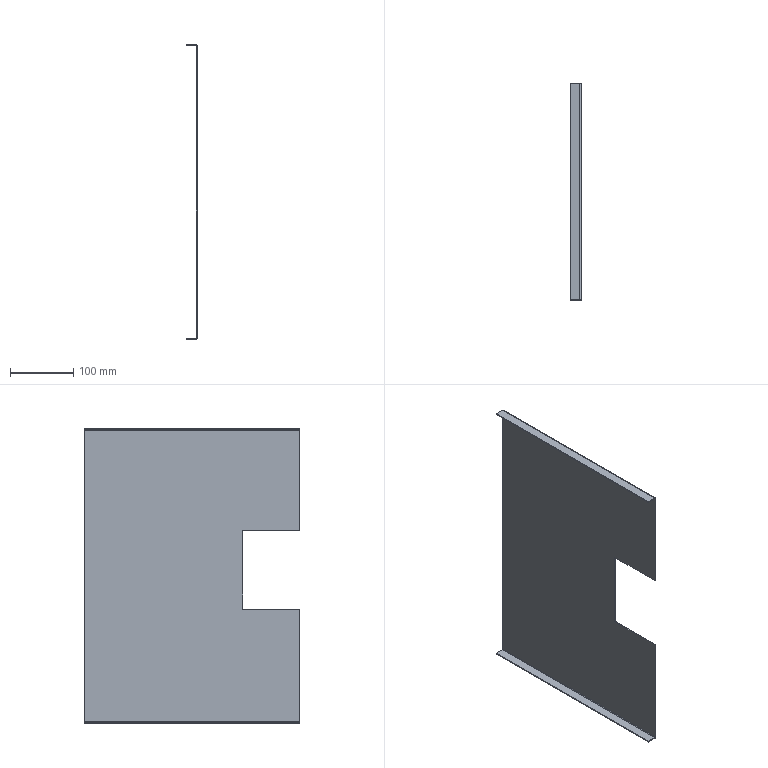Part | SolidWorks | features BaseBody 1 | 1 solid | 18 faces | box 16.5 x 340 x 464 mm | volume 234549 mm3 | plane 14 | cylinder 4 | commonest cylinder face diameters 1.473 x2 4.473 x2
STEP:
#1=CARTESIAN_POINT('',(0.,0.,-460.263));
#2=VERTEX_POINT('',#1);
#3=CARTESIAN_POINT('',(0.,0.,-282.737));
#4=VERTEX_POINT('',#3);
#5=CARTESIAN_POINT('',(0.,0.,0.));
#6=DIRECTION('',(0.,0.,1.));
#7=VECTOR('',#6,1000.);
#8=LINE('',#5,#7);
#9=EDGE_CURVE('',#2,#4,#8,.T.);
#10=ORIENTED_EDGE('',*,*,#9,.T.);
#11=CARTESIAN_POINT('',(0.,90.,-282.737));
#12=VERTEX_POINT('',#11);
#13=CARTESIAN_POINT('',(0.,340.,-282.737));
#14=DIRECTION('',(0.,1.,0.));
#15=VECTOR('',#14,1000.);
#16=LINE('',#13,#15);
#17=EDGE_CURVE('',#4,#12,#16,.T.);
#18=ORIENTED_EDGE('',*,*,#17,.T.);
#19=CARTESIAN_POINT('',(0.,90.,-158.737));
#20=VERTEX_POINT('',#19);
#21=CARTESIAN_POINT('',(0.,90.,0.));
#22=DIRECTION('',(0.,0.,1.));
#23=VECTOR('',#22,1000.);
#24=LINE('',#21,#23);
#25=EDGE_CURVE('',#12,#20,#24,.T.);
#26=ORIENTED_EDGE('',*,*,#25,.T.);
#27=CARTESIAN_POINT('',(0.,0.,-158.737));
#28=VERTEX_POINT('',#27);
#29=CARTESIAN_POINT('',(0.,340.,-158.737));
#30=DIRECTION('',(0.,-1.,0.));
#31=VECTOR('',#30,1000.);
#32=LINE('',#29,#31);
#33=EDGE_CURVE('',#20,#28,#32,.T.);
#34=ORIENTED_EDGE('',*,*,#33,.T.);
#35=CARTESIAN_POINT('',(0.,0.,-0.7366));
#36=VERTEX_POINT('',#35);
#37=CARTESIAN_POINT('',(0.,0.,0.));
#38=DIRECTION('',(0.,0.,1.));
#39=VECTOR('',#38,1000.);
#40=LINE('',#37,#39);
#41=EDGE_CURVE('',#28,#36,#40,.T.);
#42=ORIENTED_EDGE('',*,*,#41,.T.);
#43=CARTESIAN_POINT('',(0.,340.,-0.7366));
#44=VERTEX_POINT('',#43);
#45=CARTESIAN_POINT('',(0.,340.,-0.7366));
#46=DIRECTION('',(0.,1.,0.));
#47=VECTOR('',#46,1000.);
#48=LINE('',#45,#47);
#49=EDGE_CURVE('',#36,#44,#48,.T.);
#50=ORIENTED_EDGE('',*,*,#49,.T.);
#51=CARTESIAN_POINT('',(0.,340.,-460.263));
#52=VERTEX_POINT('',#51);
#53=CARTESIAN_POINT('',(0.,340.,0.));
#54=DIRECTION('',(0.,0.,-1.));
#55=VECTOR('',#54,1000.);
#56=LINE('',#53,#55);
#57=EDGE_CURVE('',#44,#52,#56,.T.);
#58=ORIENTED_EDGE('',*,*,#57,.T.);
#59=CARTESIAN_POINT('',(0.,340.,-460.263));
#60=DIRECTION('',(0.,-1.,0.));
#61=VECTOR('',#60,1000.);
#62=LINE('',#59,#61);
#63=EDGE_CURVE('',#52,#2,#62,.T.);
#64=ORIENTED_EDGE('',*,*,#63,.T.);
#65=EDGE_LOOP('',(#10,#18,#26,#34,#42,#50,#58,#64));
#66=FACE_OUTER_BOUND('',#65,.T.);
#67=CARTESIAN_POINT('',(0.,340.,0.));
#68=DIRECTION('',(-1.,0.,0.));
#69=DIRECTION('',(0.,0.,1.));
#70=AXIS2_PLACEMENT_3D('',#67,#68,#69);
#71=PLANE('',#70);
#72=ADVANCED_FACE('',(#66),#71,.T.);
#73=CARTESIAN_POINT('',(1.5,0.,-282.737));
#74=VERTEX_POINT('',#73);
#75=CARTESIAN_POINT('',(-8.5,0.,-282.737));
#76=DIRECTION('',(-1.,0.,0.));
#77=VECTOR('',#76,1000.);
#78=LINE('',#75,#77);
#79=EDGE_CURVE('',#74,#4,#78,.T.);
#80=ORIENTED_EDGE('',*,*,#79,.F.);
#81=CARTESIAN_POINT('',(1.5,90.,-282.737));
#82=VERTEX_POINT('',#81);
#83=CARTESIAN_POINT('',(1.5,0.,-282.737));
#84=DIRECTION('',(0.,-1.,0.));
#85=VECTOR('',#84,1000.);
#86=LINE('',#83,#85);
#87=EDGE_CURVE('',#82,#74,#86,.T.);
#88=ORIENTED_EDGE('',*,*,#87,.F.);
#89=CARTESIAN_POINT('',(-8.5,90.,-282.737));
#90=DIRECTION('',(1.,0.,0.));
#91=VECTOR('',#90,1000.);
#92=LINE('',#89,#91);
#93=EDGE_CURVE('',#12,#82,#92,.T.);
#94=ORIENTED_EDGE('',*,*,#93,.F.);
#95=ORIENTED_EDGE('',*,*,#17,.F.);
#96=EDGE_LOOP('',(#80,#88,#94,#95));
#97=FACE_OUTER_BOUND('',#96,.T.);
#98=CARTESIAN_POINT('',(-8.5,0.,-282.737));
#99=DIRECTION('',(0.,0.,-1.));
#100=DIRECTION('',(-1.,0.,0.));
#101=AXIS2_PLACEMENT_3D('',#98,#99,#100);
#102=PLANE('',#101);
#103=ADVANCED_FACE('',(#97),#102,.F.);
#104=ORIENTED_EDGE('',*,*,#9,.F.);
#105=CARTESIAN_POINT('',(-0.7366,0.,-461.));
#106=VERTEX_POINT('',#105);
#107=CARTESIAN_POINT('',(-0.7366,0.,-460.263));
#108=DIRECTION('',(0.,1.,0.));
#109=DIRECTION('',(0.,0.,-1.));
#110=AXIS2_PLACEMENT_3D('',#107,#108,#109);
#111=CIRCLE('',#110,0.7366);
#112=EDGE_CURVE('',#2,#106,#111,.T.);
#113=ORIENTED_EDGE('',*,*,#112,.T.);
#114=CARTESIAN_POINT('',(-15.,0.,-461.));
#115=VERTEX_POINT('',#114);
#116=CARTESIAN_POINT('',(0.,0.,-461.));
#117=DIRECTION('',(1.,0.,0.));
#118=VECTOR('',#117,1000.);
#119=LINE('',#116,#118);
#120=EDGE_CURVE('',#115,#106,#119,.T.);
#121=ORIENTED_EDGE('',*,*,#120,.F.);
#122=CARTESIAN_POINT('',(-15.,0.,-462.5));
#123=VERTEX_POINT('',#122);
#124=CARTESIAN_POINT('',(-15.,0.,-461.));
#125=DIRECTION('',(0.,0.,1.));
#126=VECTOR('',#125,1000.);
#127=LINE('',#124,#126);
#128=EDGE_CURVE('',#123,#115,#127,.T.);
#129=ORIENTED_EDGE('',*,*,#128,.F.);
#130=CARTESIAN_POINT('',(-0.7366,0.,-462.5));
#131=VERTEX_POINT('',#130);
#132=CARTESIAN_POINT('',(-0.7366,0.,-462.5));
#133=DIRECTION('',(1.,0.,0.));
#134=VECTOR('',#133,1000.);
#135=LINE('',#132,#134);
#136=EDGE_CURVE('',#123,#131,#135,.T.);
#137=ORIENTED_EDGE('',*,*,#136,.T.);
#138=CARTESIAN_POINT('',(1.5,0.,-460.263));
#139=VERTEX_POINT('',#138);
#140=CARTESIAN_POINT('',(-0.7366,0.,-460.263));
#141=DIRECTION('',(0.,1.,0.));
#142=DIRECTION('',(0.,0.,-1.));
#143=AXIS2_PLACEMENT_3D('',#140,#141,#142);
#144=CIRCLE('',#143,2.237);
#145=EDGE_CURVE('',#139,#131,#144,.T.);
#146=ORIENTED_EDGE('',*,*,#145,.F.);
#147=CARTESIAN_POINT('',(1.5,0.,-462.5));
#148=DIRECTION('',(0.,0.,1.));
#149=VECTOR('',#148,1000.);
#150=LINE('',#147,#149);
#151=EDGE_CURVE('',#139,#74,#150,.T.);
#152=ORIENTED_EDGE('',*,*,#151,.T.);
#153=ORIENTED_EDGE('',*,*,#79,.T.);
#154=EDGE_LOOP('',(#104,#113,#121,#129,#137,#146,#152,#153));
#155=FACE_OUTER_BOUND('',#154,.T.);
#156=CARTESIAN_POINT('',(-0.7366,0.,-462.5));
#157=DIRECTION('',(0.,-1.,0.));
#158=DIRECTION('',(0.,0.,-1.));
#159=AXIS2_PLACEMENT_3D('',#156,#157,#158);
#160=PLANE('',#159);
#161=ADVANCED_FACE('',(#155),#160,.T.);
#162=ORIENTED_EDGE('',*,*,#63,.F.);
#163=CARTESIAN_POINT('',(-0.7366,340.,-461.));
#164=VERTEX_POINT('',#163);
#165=CARTESIAN_POINT('',(-0.7366,340.,-460.263));
#166=DIRECTION('',(0.,-1.,0.));
#167=DIRECTION('',(0.,0.,-1.));
#168=AXIS2_PLACEMENT_3D('',#165,#166,#167);
#169=CIRCLE('',#168,0.7366);
#170=EDGE_CURVE('',#164,#52,#169,.T.);
#171=ORIENTED_EDGE('',*,*,#170,.F.);
#172=CARTESIAN_POINT('',(-0.7366,340.,-461.));
#173=DIRECTION('',(0.,1.,0.));
#174=VECTOR('',#173,1000.);
#175=LINE('',#172,#174);
#176=EDGE_CURVE('',#106,#164,#175,.T.);
#177=ORIENTED_EDGE('',*,*,#176,.F.);
#178=ORIENTED_EDGE('',*,*,#112,.F.);
#179=EDGE_LOOP('',(#162,#171,#177,#178));
#180=FACE_OUTER_BOUND('',#179,.T.);
#181=CARTESIAN_POINT('',(-0.7366,340.,-460.263));
#182=DIRECTION('',(0.,-1.,0.));
#183=DIRECTION('',(0.,0.,-1.));
#184=AXIS2_PLACEMENT_3D('',#181,#182,#183);
#185=CYLINDRICAL_SURFACE('',#184,0.7366);
#186=ADVANCED_FACE('',(#180),#185,.F.);
#187=CARTESIAN_POINT('',(1.5,340.,-0.7366));
#188=VERTEX_POINT('',#187);
#189=CARTESIAN_POINT('',(1.5,340.,-460.263));
#190=VERTEX_POINT('',#189);
#191=CARTESIAN_POINT('',(1.5,340.,1.5));
#192=DIRECTION('',(0.,0.,-1.));
#193=VECTOR('',#192,1000.);
#194=LINE('',#191,#193);
#195=EDGE_CURVE('',#188,#190,#194,.T.);
#196=ORIENTED_EDGE('',*,*,#195,.T.);
#197=CARTESIAN_POINT('',(-0.7366,340.,-462.5));
#198=VERTEX_POINT('',#197);
#199=CARTESIAN_POINT('',(-0.7366,340.,-460.263));
#200=DIRECTION('',(0.,-1.,0.));
#201=DIRECTION('',(0.,0.,-1.));
#202=AXIS2_PLACEMENT_3D('',#199,#200,#201);
#203=CIRCLE('',#202,2.237);
#204=EDGE_CURVE('',#198,#190,#203,.T.);
#205=ORIENTED_EDGE('',*,*,#204,.F.);
#206=CARTESIAN_POINT('',(-15.,340.,-462.5));
#207=VERTEX_POINT('',#206);
#208=CARTESIAN_POINT('',(1.5,340.,-462.5));
#209=DIRECTION('',(-1.,0.,0.));
#210=VECTOR('',#209,1000.);
#211=LINE('',#208,#210);
#212=EDGE_CURVE('',#198,#207,#211,.T.);
#213=ORIENTED_EDGE('',*,*,#212,.T.);
#214=CARTESIAN_POINT('',(-15.,340.,-461.));
#215=VERTEX_POINT('',#214);
#216=CARTESIAN_POINT('',(-15.,340.,-461.));
#217=DIRECTION('',(0.,0.,-1.));
#218=VECTOR('',#217,1000.);
#219=LINE('',#216,#218);
#220=EDGE_CURVE('',#215,#207,#219,.T.);
#221=ORIENTED_EDGE('',*,*,#220,.F.);
#222=CARTESIAN_POINT('',(0.,340.,-461.));
#223=DIRECTION('',(-1.,0.,0.));
#224=VECTOR('',#223,1000.);
#225=LINE('',#222,#224);
#226=EDGE_CURVE('',#164,#215,#225,.T.);
#227=ORIENTED_EDGE('',*,*,#226,.F.);
#228=ORIENTED_EDGE('',*,*,#170,.T.);
#229=ORIENTED_EDGE('',*,*,#57,.F.);
#230=CARTESIAN_POINT('',(-0.7366,340.,0.));
#231=VERTEX_POINT('',#230);
#232=CARTESIAN_POINT('',(-0.7366,340.,-0.7366));
#233=DIRECTION('',(0.,-1.,0.));
#234=DIRECTION('',(0.,0.,-1.));
#235=AXIS2_PLACEMENT_3D('',#232,#233,#234);
#236=CIRCLE('',#235,0.7366);
#237=EDGE_CURVE('',#44,#231,#236,.T.);
#238=ORIENTED_EDGE('',*,*,#237,.T.);
#239=CARTESIAN_POINT('',(-15.,340.,0.));
#240=VERTEX_POINT('',#239);
#241=CARTESIAN_POINT('',(-15.,340.,0.));
#242=DIRECTION('',(1.,0.,0.));
#243=VECTOR('',#242,1000.);
#244=LINE('',#241,#243);
#245=EDGE_CURVE('',#240,#231,#244,.T.);
#246=ORIENTED_EDGE('',*,*,#245,.F.);
#247=CARTESIAN_POINT('',(-15.,340.,1.5));
#248=VERTEX_POINT('',#247);
#249=CARTESIAN_POINT('',(-15.,340.,-460.263));
#250=DIRECTION('',(0.,0.,-1.));
#251=VECTOR('',#250,1000.);
#252=LINE('',#249,#251);
#253=EDGE_CURVE('',#248,#240,#252,.T.);
#254=ORIENTED_EDGE('',*,*,#253,.F.);
#255=CARTESIAN_POINT('',(-0.7366,340.,1.5));
#256=VERTEX_POINT('',#255);
#257=CARTESIAN_POINT('',(-0.7366,340.,1.5));
#258=DIRECTION('',(-1.,0.,0.));
#259=VECTOR('',#258,1000.);
#260=LINE('',#257,#259);
#261=EDGE_CURVE('',#256,#248,#260,.T.);
#262=ORIENTED_EDGE('',*,*,#261,.F.);
#263=CARTESIAN_POINT('',(-0.7366,340.,-0.7366));
#264=DIRECTION('',(0.,-1.,0.));
#265=DIRECTION('',(0.,0.,-1.));
#266=AXIS2_PLACEMENT_3D('',#263,#264,#265);
#267=CIRCLE('',#266,2.237);
#268=EDGE_CURVE('',#188,#256,#267,.T.);
#269=ORIENTED_EDGE('',*,*,#268,.F.);
#270=EDGE_LOOP('',(#196,#205,#213,#221,#227,#228,#229,#238,#246,#254,#262,#269));
#271=FACE_OUTER_BOUND('',#270,.T.);
#272=CARTESIAN_POINT('',(-0.7366,340.,1.5));
#273=DIRECTION('',(0.,1.,0.));
#274=DIRECTION('',(0.,0.,1.));
#275=AXIS2_PLACEMENT_3D('',#272,#273,#274);
#276=PLANE('',#275);
#277=ADVANCED_FACE('',(#271),#276,.T.);
#278=CARTESIAN_POINT('',(-0.7366,0.,0.));
#279=VERTEX_POINT('',#278);
#280=CARTESIAN_POINT('',(-0.7366,340.,0.));
#281=DIRECTION('',(0.,-1.,0.));
#282=VECTOR('',#281,1000.);
#283=LINE('',#280,#282);
#284=EDGE_CURVE('',#231,#279,#283,.T.);
#285=ORIENTED_EDGE('',*,*,#284,.F.);
#286=ORIENTED_EDGE('',*,*,#237,.F.);
#287=ORIENTED_EDGE('',*,*,#49,.F.);
#288=CARTESIAN_POINT('',(-0.7366,0.,-0.7366));
#289=DIRECTION('',(0.,1.,0.));
#290=DIRECTION('',(0.,0.,-1.));
#291=AXIS2_PLACEMENT_3D('',#288,#289,#290);
#292=CIRCLE('',#291,0.7366);
#293=EDGE_CURVE('',#279,#36,#292,.T.);
#294=ORIENTED_EDGE('',*,*,#293,.F.);
#295=EDGE_LOOP('',(#285,#286,#287,#294));
#296=FACE_OUTER_BOUND('',#295,.T.);
#297=CARTESIAN_POINT('',(-0.7366,340.,-0.7366));
#298=DIRECTION('',(0.,-1.,0.));
#299=DIRECTION('',(0.,0.,-1.));
#300=AXIS2_PLACEMENT_3D('',#297,#298,#299);
#301=CYLINDRICAL_SURFACE('',#300,0.7366);
#302=ADVANCED_FACE('',(#296),#301,.F.);
#303=CARTESIAN_POINT('',(1.5,0.,-158.737));
#304=VERTEX_POINT('',#303);
#305=CARTESIAN_POINT('',(1.5,0.,-0.7366));
#306=VERTEX_POINT('',#305);
#307=CARTESIAN_POINT('',(1.5,0.,-462.5));
#308=DIRECTION('',(0.,0.,1.));
#309=VECTOR('',#308,1000.);
#310=LINE('',#307,#309);
#311=EDGE_CURVE('',#304,#306,#310,.T.);
#312=ORIENTED_EDGE('',*,*,#311,.T.);
#313=CARTESIAN_POINT('',(-0.7366,0.,1.5));
#314=VERTEX_POINT('',#313);
#315=CARTESIAN_POINT('',(-0.7366,0.,-0.7366));
#316=DIRECTION('',(0.,1.,0.));
#317=DIRECTION('',(0.,0.,-1.));
#318=AXIS2_PLACEMENT_3D('',#315,#316,#317);
#319=CIRCLE('',#318,2.237);
#320=EDGE_CURVE('',#314,#306,#319,.T.);
#321=ORIENTED_EDGE('',*,*,#320,.F.);
#322=CARTESIAN_POINT('',(-15.,0.,1.5));
#323=VERTEX_POINT('',#322);
#324=CARTESIAN_POINT('',(1.5,0.,1.5));
#325=DIRECTION('',(-1.,0.,0.));
#326=VECTOR('',#325,1000.);
#327=LINE('',#324,#326);
#328=EDGE_CURVE('',#314,#323,#327,.T.);
#329=ORIENTED_EDGE('',*,*,#328,.T.);
#330=CARTESIAN_POINT('',(-15.,0.,0.));
#331=VERTEX_POINT('',#330);
#332=CARTESIAN_POINT('',(-15.,0.,1.5));
#333=DIRECTION('',(0.,0.,1.));
#334=VECTOR('',#333,1000.);
#335=LINE('',#332,#334);
#336=EDGE_CURVE('',#331,#323,#335,.T.);
#337=ORIENTED_EDGE('',*,*,#336,.F.);
#338=CARTESIAN_POINT('',(-15.,0.,0.));
#339=DIRECTION('',(-1.,0.,0.));
#340=VECTOR('',#339,1000.);
#341=LINE('',#338,#340);
#342=EDGE_CURVE('',#279,#331,#341,.T.);
#343=ORIENTED_EDGE('',*,*,#342,.F.);
#344=ORIENTED_EDGE('',*,*,#293,.T.);
#345=ORIENTED_EDGE('',*,*,#41,.F.);
#346=CARTESIAN_POINT('',(-0.7366,0.,-158.737));
#347=DIRECTION('',(1.,0.,0.));
#348=VECTOR('',#347,1000.);
#349=LINE('',#346,#348);
#350=EDGE_CURVE('',#28,#304,#349,.T.);
#351=ORIENTED_EDGE('',*,*,#350,.T.);
#352=EDGE_LOOP('',(#312,#321,#329,#337,#343,#344,#345,#351));
#353=FACE_OUTER_BOUND('',#352,.T.);
#354=CARTESIAN_POINT('',(-0.7366,0.,-462.5));
#355=DIRECTION('',(0.,-1.,0.));
#356=DIRECTION('',(0.,0.,-1.));
#357=AXIS2_PLACEMENT_3D('',#354,#355,#356);
#358=PLANE('',#357);
#359=ADVANCED_FACE('',(#353),#358,.T.);
#360=ORIENTED_EDGE('',*,*,#350,.F.);
#361=ORIENTED_EDGE('',*,*,#33,.F.);
#362=CARTESIAN_POINT('',(1.5,90.,-158.737));
#363=VERTEX_POINT('',#362);
#364=CARTESIAN_POINT('',(-8.5,90.,-158.737));
#365=DIRECTION('',(1.,0.,0.));
#366=VECTOR('',#365,1000.);
#367=LINE('',#364,#366);
#368=EDGE_CURVE('',#20,#363,#367,.T.);
#369=ORIENTED_EDGE('',*,*,#368,.T.);
#370=CARTESIAN_POINT('',(1.5,0.,-158.737));
#371=DIRECTION('',(0.,-1.,0.));
#372=VECTOR('',#371,1000.);
#373=LINE('',#370,#372);
#374=EDGE_CURVE('',#363,#304,#373,.T.);
#375=ORIENTED_EDGE('',*,*,#374,.T.);
#376=EDGE_LOOP('',(#360,#361,#369,#375));
#377=FACE_OUTER_BOUND('',#376,.T.);
#378=CARTESIAN_POINT('',(-8.5,0.,-158.737));
#379=DIRECTION('',(0.,0.,-1.));
#380=DIRECTION('',(-1.,0.,0.));
#381=AXIS2_PLACEMENT_3D('',#378,#379,#380);
#382=PLANE('',#381);
#383=ADVANCED_FACE('',(#377),#382,.T.);
#384=ORIENTED_EDGE('',*,*,#368,.F.);
#385=ORIENTED_EDGE('',*,*,#25,.F.);
#386=ORIENTED_EDGE('',*,*,#93,.T.);
#387=CARTESIAN_POINT('',(1.5,90.,-158.737));
#388=DIRECTION('',(0.,0.,1.));
#389=VECTOR('',#388,1000.);
#390=LINE('',#387,#389);
#391=EDGE_CURVE('',#82,#363,#390,.T.);
#392=ORIENTED_EDGE('',*,*,#391,.T.);
#393=EDGE_LOOP('',(#384,#385,#386,#392));
#394=FACE_OUTER_BOUND('',#393,.T.);
#395=CARTESIAN_POINT('',(-8.5,90.,-158.737));
#396=DIRECTION('',(0.,-1.,0.));
#397=DIRECTION('',(0.,0.,-1.));
#398=AXIS2_PLACEMENT_3D('',#395,#396,#397);
#399=PLANE('',#398);
#400=ADVANCED_FACE('',(#394),#399,.T.);
#401=ORIENTED_EDGE('',*,*,#391,.F.);
#402=ORIENTED_EDGE('',*,*,#87,.T.);
#403=ORIENTED_EDGE('',*,*,#151,.F.);
#404=CARTESIAN_POINT('',(1.5,340.,-460.263));
#405=DIRECTION('',(0.,-1.,0.));
#406=VECTOR('',#405,1000.);
#407=LINE('',#404,#406);
#408=EDGE_CURVE('',#190,#139,#407,.T.);
#409=ORIENTED_EDGE('',*,*,#408,.F.);
#410=ORIENTED_EDGE('',*,*,#195,.F.);
#411=CARTESIAN_POINT('',(1.5,340.,-0.7366));
#412=DIRECTION('',(0.,1.,0.));
#413=VECTOR('',#412,1000.);
#414=LINE('',#411,#413);
#415=EDGE_CURVE('',#306,#188,#414,.T.);
#416=ORIENTED_EDGE('',*,*,#415,.F.);
#417=ORIENTED_EDGE('',*,*,#311,.F.);
#418=ORIENTED_EDGE('',*,*,#374,.F.);
#419=EDGE_LOOP('',(#401,#402,#403,#409,#410,#416,#417,#418));
#420=FACE_OUTER_BOUND('',#419,.T.);
#421=CARTESIAN_POINT('',(1.5,340.,0.));
#422=DIRECTION('',(-1.,0.,0.));
#423=DIRECTION('',(0.,0.,1.));
#424=AXIS2_PLACEMENT_3D('',#421,#422,#423);
#425=PLANE('',#424);
#426=ADVANCED_FACE('',(#420),#425,.F.);
#427=ORIENTED_EDGE('',*,*,#226,.T.);
#428=CARTESIAN_POINT('',(-15.,340.,-461.));
#429=DIRECTION('',(0.,-1.,0.));
#430=VECTOR('',#429,1000.);
#431=LINE('',#428,#430);
#432=EDGE_CURVE('',#215,#115,#431,.T.);
#433=ORIENTED_EDGE('',*,*,#432,.T.);
#434=ORIENTED_EDGE('',*,*,#120,.T.);
#435=ORIENTED_EDGE('',*,*,#176,.T.);
#436=EDGE_LOOP('',(#427,#433,#434,#435));
#437=FACE_OUTER_BOUND('',#436,.T.);
#438=CARTESIAN_POINT('',(0.,340.,-461.));
#439=DIRECTION('',(0.,0.,1.));
#440=DIRECTION('',(1.,0.,0.));
#441=AXIS2_PLACEMENT_3D('',#438,#439,#440);
#442=PLANE('',#441);
#443=ADVANCED_FACE('',(#437),#442,.T.);
#444=ORIENTED_EDGE('',*,*,#245,.T.);
#445=ORIENTED_EDGE('',*,*,#284,.T.);
#446=ORIENTED_EDGE('',*,*,#342,.T.);
#447=CARTESIAN_POINT('',(-15.,340.,0.));
#448=DIRECTION('',(0.,1.,0.));
#449=VECTOR('',#448,1000.);
#450=LINE('',#447,#449);
#451=EDGE_CURVE('',#331,#240,#450,.T.);
#452=ORIENTED_EDGE('',*,*,#451,.T.);
#453=EDGE_LOOP('',(#444,#445,#446,#452));
#454=FACE_OUTER_BOUND('',#453,.T.);
#455=CARTESIAN_POINT('',(-15.,340.,0.));
#456=DIRECTION('',(0.,0.,-1.));
#457=DIRECTION('',(-1.,0.,0.));
#458=AXIS2_PLACEMENT_3D('',#455,#456,#457);
#459=PLANE('',#458);
#460=ADVANCED_FACE('',(#454),#459,.T.);
#461=ORIENTED_EDGE('',*,*,#204,.T.);
#462=ORIENTED_EDGE('',*,*,#408,.T.);
#463=ORIENTED_EDGE('',*,*,#145,.T.);
#464=CARTESIAN_POINT('',(-0.7366,340.,-462.5));
#465=DIRECTION('',(0.,1.,0.));
#466=VECTOR('',#465,1000.);
#467=LINE('',#464,#466);
#468=EDGE_CURVE('',#131,#198,#467,.T.);
#469=ORIENTED_EDGE('',*,*,#468,.T.);
#470=EDGE_LOOP('',(#461,#462,#463,#469));
#471=FACE_OUTER_BOUND('',#470,.T.);
#472=CARTESIAN_POINT('',(-0.7366,340.,-460.263));
#473=DIRECTION('',(0.,-1.,0.));
#474=DIRECTION('',(0.,0.,-1.));
#475=AXIS2_PLACEMENT_3D('',#472,#473,#474);
#476=CYLINDRICAL_SURFACE('',#475,2.237);
#477=ADVANCED_FACE('',(#471),#476,.T.);
#478=ORIENTED_EDGE('',*,*,#268,.T.);
#479=CARTESIAN_POINT('',(-0.7366,340.,1.5));
#480=DIRECTION('',(0.,-1.,0.));
#481=VECTOR('',#480,1000.);
#482=LINE('',#479,#481);
#483=EDGE_CURVE('',#256,#314,#482,.T.);
#484=ORIENTED_EDGE('',*,*,#483,.T.);
#485=ORIENTED_EDGE('',*,*,#320,.T.);
#486=ORIENTED_EDGE('',*,*,#415,.T.);
#487=EDGE_LOOP('',(#478,#484,#485,#486));
#488=FACE_OUTER_BOUND('',#487,.T.);
#489=CARTESIAN_POINT('',(-0.7366,340.,-0.7366));
#490=DIRECTION('',(0.,-1.,0.));
#491=DIRECTION('',(0.,0.,-1.));
#492=AXIS2_PLACEMENT_3D('',#489,#490,#491);
#493=CYLINDRICAL_SURFACE('',#492,2.237);
#494=ADVANCED_FACE('',(#488),#493,.T.);
#495=ORIENTED_EDGE('',*,*,#220,.T.);
#496=CARTESIAN_POINT('',(-15.,340.,-462.5));
#497=DIRECTION('',(0.,-1.,0.));
#498=VECTOR('',#497,1000.);
#499=LINE('',#496,#498);
#500=EDGE_CURVE('',#207,#123,#499,.T.);
#501=ORIENTED_EDGE('',*,*,#500,.T.);
#502=ORIENTED_EDGE('',*,*,#128,.T.);
#503=ORIENTED_EDGE('',*,*,#432,.F.);
#504=EDGE_LOOP('',(#495,#501,#502,#503));
#505=FACE_OUTER_BOUND('',#504,.T.);
#506=CARTESIAN_POINT('',(-15.,340.,-461.));
#507=DIRECTION('',(-1.,0.,0.));
#508=DIRECTION('',(0.,0.,1.));
#509=AXIS2_PLACEMENT_3D('',#506,#507,#508);
#510=PLANE('',#509);
#511=ADVANCED_FACE('',(#505),#510,.T.);
#512=ORIENTED_EDGE('',*,*,#253,.T.);
#513=ORIENTED_EDGE('',*,*,#451,.F.);
#514=ORIENTED_EDGE('',*,*,#336,.T.);
#515=CARTESIAN_POINT('',(-15.,340.,1.5));
#516=DIRECTION('',(0.,1.,0.));
#517=VECTOR('',#516,1000.);
#518=LINE('',#515,#517);
#519=EDGE_CURVE('',#323,#248,#518,.T.);
#520=ORIENTED_EDGE('',*,*,#519,.T.);
#521=EDGE_LOOP('',(#512,#513,#514,#520));
#522=FACE_OUTER_BOUND('',#521,.T.);
#523=CARTESIAN_POINT('',(-15.,340.,1.5));
#524=DIRECTION('',(-1.,0.,0.));
#525=DIRECTION('',(0.,0.,1.));
#526=AXIS2_PLACEMENT_3D('',#523,#524,#525);
#527=PLANE('',#526);
#528=ADVANCED_FACE('',(#522),#527,.T.);
#529=ORIENTED_EDGE('',*,*,#500,.F.);
#530=ORIENTED_EDGE('',*,*,#212,.F.);
#531=ORIENTED_EDGE('',*,*,#468,.F.);
#532=ORIENTED_EDGE('',*,*,#136,.F.);
#533=EDGE_LOOP('',(#529,#530,#531,#532));
#534=FACE_OUTER_BOUND('',#533,.T.);
#535=CARTESIAN_POINT('',(0.,340.,-462.5));
#536=DIRECTION('',(0.,0.,1.));
#537=DIRECTION('',(1.,0.,0.));
#538=AXIS2_PLACEMENT_3D('',#535,#536,#537);
#539=PLANE('',#538);
#540=ADVANCED_FACE('',(#534),#539,.F.);
#541=ORIENTED_EDGE('',*,*,#483,.F.);
#542=ORIENTED_EDGE('',*,*,#261,.T.);
#543=ORIENTED_EDGE('',*,*,#519,.F.);
#544=ORIENTED_EDGE('',*,*,#328,.F.);
#545=EDGE_LOOP('',(#541,#542,#543,#544));
#546=FACE_OUTER_BOUND('',#545,.T.);
#547=CARTESIAN_POINT('',(-15.,340.,1.5));
#548=DIRECTION('',(0.,0.,-1.));
#549=DIRECTION('',(-1.,0.,0.));
#550=AXIS2_PLACEMENT_3D('',#547,#548,#549);
#551=PLANE('',#550);
#552=ADVANCED_FACE('',(#546),#551,.F.);
#553=CLOSED_SHELL('',(#72,#103,#161,#186,#277,#302,#359,#383,#400,#426,#443,#460,#477,#494,#511,#528,#540,#552));
#554=MANIFOLD_SOLID_BREP('',#553);
#555=CARTESIAN_POINT('',(0.,0.,0.));
#556=DIRECTION('',(0.,0.,1.));
#557=DIRECTION('',(1.,0.,0.));
#558=AXIS2_PLACEMENT_3D('',#555,#556,#557);
#559=(LENGTH_UNIT()NAMED_UNIT(*)SI_UNIT(.MILLI.,.METRE.));
#560=UNCERTAINTY_MEASURE_WITH_UNIT(LENGTH_MEASURE(0.00001),#559,'','');
#561=(NAMED_UNIT(*)PLANE_ANGLE_UNIT()SI_UNIT($,.RADIAN.));
#562=(NAMED_UNIT(*)SI_UNIT($,.STERADIAN.)SOLID_ANGLE_UNIT());
#563=(GEOMETRIC_REPRESENTATION_CONTEXT(3)GLOBAL_UNCERTAINTY_ASSIGNED_CONTEXT((#560))GLOBAL_UNIT_ASSIGNED_CONTEXT((#559,#561,#562))REPRESENTATION_CONTEXT('',''));
#564=ADVANCED_BREP_SHAPE_REPRESENTATION('',(#554,#558),#563);